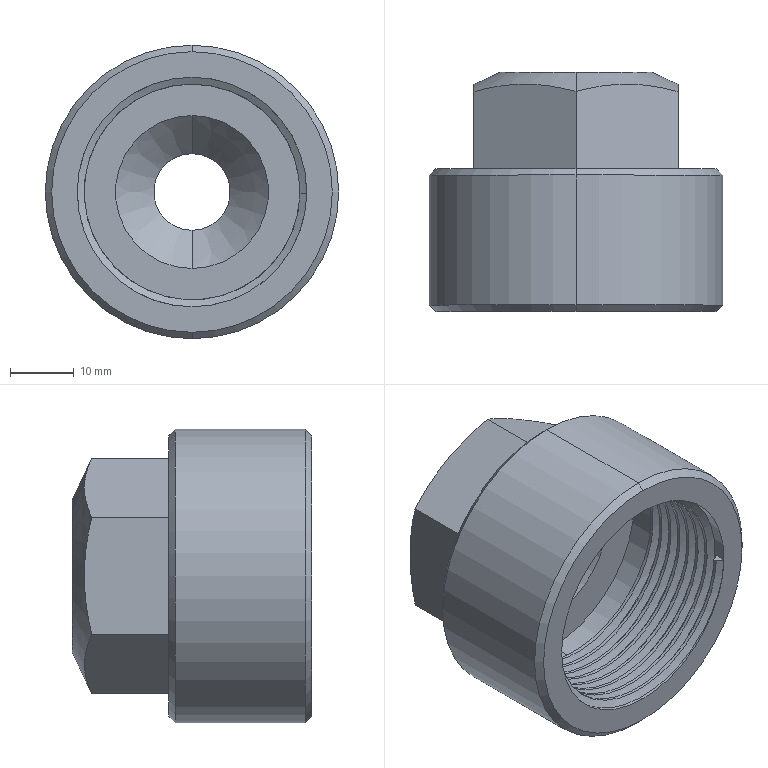Part | SolidWorks | features Chamfer 1, ICE 1, Revolution 1, SweepThread 1 | 1 solid | 48 faces | box 46 x 37.5 x 46 mm | volume 24273 mm3 | cylinder 23 | plane 12 | cone 10 | spline 3 | commonest cylinder face diameters 36 x17 12 x2 24 x2 46 x2